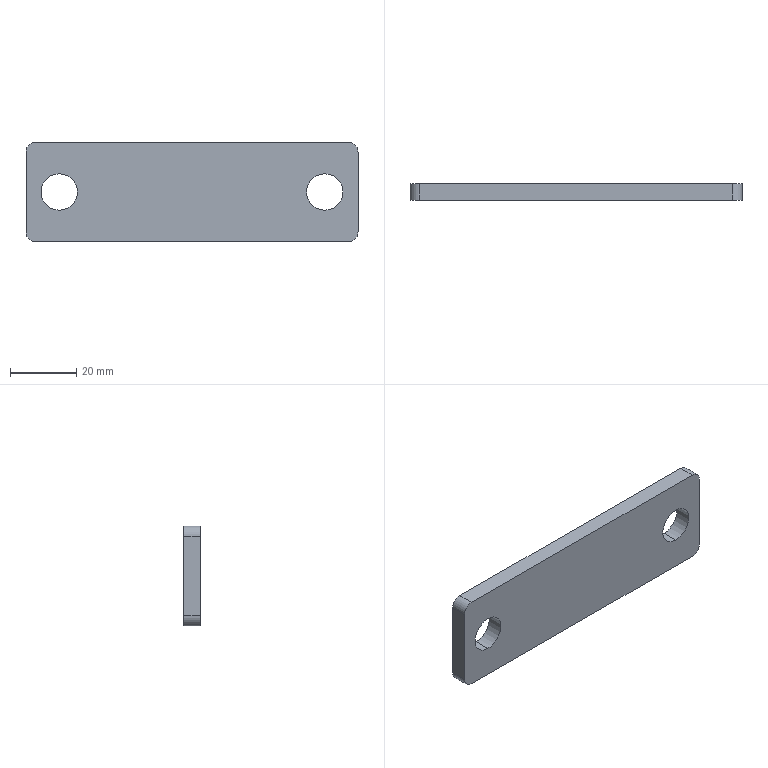Part | SolidWorks | features Extrusion 1, Fillet 1, ICE 1 | 1 solid | 14 faces | box 100 x 5 x 30 mm | volume 14011 mm3 | cylinder 8 | plane 6 | commonest cylinder face diameters 6 x4 11 x4
STEP:
#1=CARTESIAN_POINT('',(-40.,0.,5.5));
#2=VERTEX_POINT('',#1);
#3=CARTESIAN_POINT('',(-40.,0.,-5.5));
#4=VERTEX_POINT('',#3);
#5=CARTESIAN_POINT('',(-40.,0.,0.));
#6=DIRECTION('',(0.,-1.,0.));
#7=DIRECTION('',(0.,0.,-1.));
#8=AXIS2_PLACEMENT_3D('',#5,#6,#7);
#9=CIRCLE('',#8,5.5);
#10=EDGE_CURVE('',#2,#4,#9,.T.);
#11=ORIENTED_EDGE('',*,*,#10,.T.);
#12=CARTESIAN_POINT('',(-40.,5.,-5.5));
#13=VERTEX_POINT('',#12);
#14=CARTESIAN_POINT('',(-40.,-5.,-5.5));
#15=DIRECTION('',(0.,1.,0.));
#16=VECTOR('',#15,1000.);
#17=LINE('',#14,#16);
#18=EDGE_CURVE('',#4,#13,#17,.T.);
#19=ORIENTED_EDGE('',*,*,#18,.T.);
#20=CARTESIAN_POINT('',(-40.,5.,5.5));
#21=VERTEX_POINT('',#20);
#22=CARTESIAN_POINT('',(-40.,5.,0.));
#23=DIRECTION('',(0.,1.,0.));
#24=DIRECTION('',(0.,0.,1.));
#25=AXIS2_PLACEMENT_3D('',#22,#23,#24);
#26=CIRCLE('',#25,5.5);
#27=EDGE_CURVE('',#13,#21,#26,.T.);
#28=ORIENTED_EDGE('',*,*,#27,.T.);
#29=CARTESIAN_POINT('',(-40.,-5.,5.5));
#30=DIRECTION('',(0.,1.,0.));
#31=VECTOR('',#30,1000.);
#32=LINE('',#29,#31);
#33=EDGE_CURVE('',#2,#21,#32,.T.);
#34=ORIENTED_EDGE('',*,*,#33,.F.);
#35=EDGE_LOOP('',(#11,#19,#28,#34));
#36=FACE_OUTER_BOUND('',#35,.T.);
#37=CARTESIAN_POINT('',(-40.,-5.,0.));
#38=DIRECTION('',(0.,1.,0.));
#39=DIRECTION('',(0.,0.,1.));
#40=AXIS2_PLACEMENT_3D('',#37,#38,#39);
#41=CYLINDRICAL_SURFACE('',#40,5.5);
#42=ADVANCED_FACE('',(#36),#41,.F.);
#43=CARTESIAN_POINT('',(40.,0.,5.5));
#44=VERTEX_POINT('',#43);
#45=CARTESIAN_POINT('',(40.,0.,-5.5));
#46=VERTEX_POINT('',#45);
#47=CARTESIAN_POINT('',(40.,0.,0.));
#48=DIRECTION('',(0.,-1.,0.));
#49=DIRECTION('',(0.,0.,-1.));
#50=AXIS2_PLACEMENT_3D('',#47,#48,#49);
#51=CIRCLE('',#50,5.5);
#52=EDGE_CURVE('',#44,#46,#51,.T.);
#53=ORIENTED_EDGE('',*,*,#52,.T.);
#54=CARTESIAN_POINT('',(40.,5.,-5.5));
#55=VERTEX_POINT('',#54);
#56=CARTESIAN_POINT('',(40.,-5.,-5.5));
#57=DIRECTION('',(0.,1.,0.));
#58=VECTOR('',#57,1000.);
#59=LINE('',#56,#58);
#60=EDGE_CURVE('',#46,#55,#59,.T.);
#61=ORIENTED_EDGE('',*,*,#60,.T.);
#62=CARTESIAN_POINT('',(40.,5.,5.5));
#63=VERTEX_POINT('',#62);
#64=CARTESIAN_POINT('',(40.,5.,0.));
#65=DIRECTION('',(0.,1.,0.));
#66=DIRECTION('',(0.,0.,1.));
#67=AXIS2_PLACEMENT_3D('',#64,#65,#66);
#68=CIRCLE('',#67,5.5);
#69=EDGE_CURVE('',#55,#63,#68,.T.);
#70=ORIENTED_EDGE('',*,*,#69,.T.);
#71=CARTESIAN_POINT('',(40.,-5.,5.5));
#72=DIRECTION('',(0.,1.,0.));
#73=VECTOR('',#72,1000.);
#74=LINE('',#71,#73);
#75=EDGE_CURVE('',#44,#63,#74,.T.);
#76=ORIENTED_EDGE('',*,*,#75,.F.);
#77=EDGE_LOOP('',(#53,#61,#70,#76));
#78=FACE_OUTER_BOUND('',#77,.T.);
#79=CARTESIAN_POINT('',(40.,-5.,0.));
#80=DIRECTION('',(0.,1.,0.));
#81=DIRECTION('',(0.,0.,1.));
#82=AXIS2_PLACEMENT_3D('',#79,#80,#81);
#83=CYLINDRICAL_SURFACE('',#82,5.5);
#84=ADVANCED_FACE('',(#78),#83,.F.);
#85=CARTESIAN_POINT('',(50.,5.,12.));
#86=VERTEX_POINT('',#85);
#87=CARTESIAN_POINT('',(50.,5.,-12.));
#88=VERTEX_POINT('',#87);
#89=CARTESIAN_POINT('',(50.,5.,15.));
#90=DIRECTION('',(0.,0.,-1.));
#91=VECTOR('',#90,1000.);
#92=LINE('',#89,#91);
#93=EDGE_CURVE('',#86,#88,#92,.T.);
#94=ORIENTED_EDGE('',*,*,#93,.F.);
#95=CARTESIAN_POINT('',(50.,0.,12.));
#96=VERTEX_POINT('',#95);
#97=CARTESIAN_POINT('',(50.,5.,12.));
#98=DIRECTION('',(0.,-1.,0.));
#99=VECTOR('',#98,1000.);
#100=LINE('',#97,#99);
#101=EDGE_CURVE('',#86,#96,#100,.T.);
#102=ORIENTED_EDGE('',*,*,#101,.T.);
#103=CARTESIAN_POINT('',(50.,0.,-12.));
#104=VERTEX_POINT('',#103);
#105=CARTESIAN_POINT('',(50.,0.,15.));
#106=DIRECTION('',(0.,0.,-1.));
#107=VECTOR('',#106,1000.);
#108=LINE('',#105,#107);
#109=EDGE_CURVE('',#96,#104,#108,.T.);
#110=ORIENTED_EDGE('',*,*,#109,.T.);
#111=CARTESIAN_POINT('',(50.,5.,-12.));
#112=DIRECTION('',(0.,1.,0.));
#113=VECTOR('',#112,1000.);
#114=LINE('',#111,#113);
#115=EDGE_CURVE('',#104,#88,#114,.T.);
#116=ORIENTED_EDGE('',*,*,#115,.T.);
#117=EDGE_LOOP('',(#94,#102,#110,#116));
#118=FACE_OUTER_BOUND('',#117,.T.);
#119=CARTESIAN_POINT('',(50.,5.,15.));
#120=DIRECTION('',(-1.,0.,0.));
#121=DIRECTION('',(0.,0.,1.));
#122=AXIS2_PLACEMENT_3D('',#119,#120,#121);
#123=PLANE('',#122);
#124=ADVANCED_FACE('',(#118),#123,.F.);
#125=CARTESIAN_POINT('',(47.,5.,-15.));
#126=VERTEX_POINT('',#125);
#127=CARTESIAN_POINT('',(-47.,5.,-15.));
#128=VERTEX_POINT('',#127);
#129=CARTESIAN_POINT('',(-50.,5.,-15.));
#130=DIRECTION('',(-1.,0.,0.));
#131=VECTOR('',#130,1000.);
#132=LINE('',#129,#131);
#133=EDGE_CURVE('',#126,#128,#132,.T.);
#134=ORIENTED_EDGE('',*,*,#133,.F.);
#135=CARTESIAN_POINT('',(47.,0.,-15.));
#136=VERTEX_POINT('',#135);
#137=CARTESIAN_POINT('',(47.,5.,-15.));
#138=DIRECTION('',(0.,-1.,0.));
#139=VECTOR('',#138,1000.);
#140=LINE('',#137,#139);
#141=EDGE_CURVE('',#126,#136,#140,.T.);
#142=ORIENTED_EDGE('',*,*,#141,.T.);
#143=CARTESIAN_POINT('',(-47.,0.,-15.));
#144=VERTEX_POINT('',#143);
#145=CARTESIAN_POINT('',(-50.,0.,-15.));
#146=DIRECTION('',(-1.,0.,0.));
#147=VECTOR('',#146,1000.);
#148=LINE('',#145,#147);
#149=EDGE_CURVE('',#136,#144,#148,.T.);
#150=ORIENTED_EDGE('',*,*,#149,.T.);
#151=CARTESIAN_POINT('',(-47.,5.,-15.));
#152=DIRECTION('',(0.,1.,0.));
#153=VECTOR('',#152,1000.);
#154=LINE('',#151,#153);
#155=EDGE_CURVE('',#144,#128,#154,.T.);
#156=ORIENTED_EDGE('',*,*,#155,.T.);
#157=EDGE_LOOP('',(#134,#142,#150,#156));
#158=FACE_OUTER_BOUND('',#157,.T.);
#159=CARTESIAN_POINT('',(-50.,5.,-15.));
#160=DIRECTION('',(0.,0.,1.));
#161=DIRECTION('',(1.,0.,0.));
#162=AXIS2_PLACEMENT_3D('',#159,#160,#161);
#163=PLANE('',#162);
#164=ADVANCED_FACE('',(#158),#163,.F.);
#165=CARTESIAN_POINT('',(-50.,5.,-12.));
#166=VERTEX_POINT('',#165);
#167=CARTESIAN_POINT('',(-50.,5.,12.));
#168=VERTEX_POINT('',#167);
#169=CARTESIAN_POINT('',(-50.,5.,15.));
#170=DIRECTION('',(0.,0.,1.));
#171=VECTOR('',#170,1000.);
#172=LINE('',#169,#171);
#173=EDGE_CURVE('',#166,#168,#172,.T.);
#174=ORIENTED_EDGE('',*,*,#173,.F.);
#175=CARTESIAN_POINT('',(-50.,0.,-12.));
#176=VERTEX_POINT('',#175);
#177=CARTESIAN_POINT('',(-50.,5.,-12.));
#178=DIRECTION('',(0.,-1.,0.));
#179=VECTOR('',#178,1000.);
#180=LINE('',#177,#179);
#181=EDGE_CURVE('',#166,#176,#180,.T.);
#182=ORIENTED_EDGE('',*,*,#181,.T.);
#183=CARTESIAN_POINT('',(-50.,0.,12.));
#184=VERTEX_POINT('',#183);
#185=CARTESIAN_POINT('',(-50.,0.,15.));
#186=DIRECTION('',(0.,0.,1.));
#187=VECTOR('',#186,1000.);
#188=LINE('',#185,#187);
#189=EDGE_CURVE('',#176,#184,#188,.T.);
#190=ORIENTED_EDGE('',*,*,#189,.T.);
#191=CARTESIAN_POINT('',(-50.,5.,12.));
#192=DIRECTION('',(0.,1.,0.));
#193=VECTOR('',#192,1000.);
#194=LINE('',#191,#193);
#195=EDGE_CURVE('',#184,#168,#194,.T.);
#196=ORIENTED_EDGE('',*,*,#195,.T.);
#197=EDGE_LOOP('',(#174,#182,#190,#196));
#198=FACE_OUTER_BOUND('',#197,.T.);
#199=CARTESIAN_POINT('',(-50.,5.,15.));
#200=DIRECTION('',(1.,0.,0.));
#201=DIRECTION('',(0.,0.,-1.));
#202=AXIS2_PLACEMENT_3D('',#199,#200,#201);
#203=PLANE('',#202);
#204=ADVANCED_FACE('',(#198),#203,.F.);
#205=CARTESIAN_POINT('',(-47.,0.,15.));
#206=VERTEX_POINT('',#205);
#207=CARTESIAN_POINT('',(47.,0.,15.));
#208=VERTEX_POINT('',#207);
#209=CARTESIAN_POINT('',(-50.,0.,15.));
#210=DIRECTION('',(1.,0.,0.));
#211=VECTOR('',#210,1000.);
#212=LINE('',#209,#211);
#213=EDGE_CURVE('',#206,#208,#212,.T.);
#214=ORIENTED_EDGE('',*,*,#213,.T.);
#215=CARTESIAN_POINT('',(47.,5.,15.));
#216=VERTEX_POINT('',#215);
#217=CARTESIAN_POINT('',(47.,5.,15.));
#218=DIRECTION('',(0.,1.,0.));
#219=VECTOR('',#218,1000.);
#220=LINE('',#217,#219);
#221=EDGE_CURVE('',#208,#216,#220,.T.);
#222=ORIENTED_EDGE('',*,*,#221,.T.);
#223=CARTESIAN_POINT('',(-47.,5.,15.));
#224=VERTEX_POINT('',#223);
#225=CARTESIAN_POINT('',(-50.,5.,15.));
#226=DIRECTION('',(1.,0.,0.));
#227=VECTOR('',#226,1000.);
#228=LINE('',#225,#227);
#229=EDGE_CURVE('',#224,#216,#228,.T.);
#230=ORIENTED_EDGE('',*,*,#229,.F.);
#231=CARTESIAN_POINT('',(-47.,5.,15.));
#232=DIRECTION('',(0.,-1.,0.));
#233=VECTOR('',#232,1000.);
#234=LINE('',#231,#233);
#235=EDGE_CURVE('',#224,#206,#234,.T.);
#236=ORIENTED_EDGE('',*,*,#235,.T.);
#237=EDGE_LOOP('',(#214,#222,#230,#236));
#238=FACE_OUTER_BOUND('',#237,.T.);
#239=CARTESIAN_POINT('',(-50.,5.,15.));
#240=DIRECTION('',(0.,0.,-1.));
#241=DIRECTION('',(-1.,0.,0.));
#242=AXIS2_PLACEMENT_3D('',#239,#240,#241);
#243=PLANE('',#242);
#244=ADVANCED_FACE('',(#238),#243,.F.);
#245=CARTESIAN_POINT('',(-40.,5.,0.));
#246=DIRECTION('',(0.,1.,0.));
#247=DIRECTION('',(0.,0.,1.));
#248=AXIS2_PLACEMENT_3D('',#245,#246,#247);
#249=CIRCLE('',#248,5.5);
#250=EDGE_CURVE('',#21,#13,#249,.T.);
#251=ORIENTED_EDGE('',*,*,#250,.F.);
#252=ORIENTED_EDGE('',*,*,#27,.F.);
#253=EDGE_LOOP('',(#251,#252));
#254=FACE_BOUND('',#253,.T.);
#255=CARTESIAN_POINT('',(40.,5.,0.));
#256=DIRECTION('',(0.,1.,0.));
#257=DIRECTION('',(0.,0.,1.));
#258=AXIS2_PLACEMENT_3D('',#255,#256,#257);
#259=CIRCLE('',#258,5.5);
#260=EDGE_CURVE('',#63,#55,#259,.T.);
#261=ORIENTED_EDGE('',*,*,#260,.F.);
#262=ORIENTED_EDGE('',*,*,#69,.F.);
#263=EDGE_LOOP('',(#261,#262));
#264=FACE_BOUND('',#263,.T.);
#265=ORIENTED_EDGE('',*,*,#229,.T.);
#266=CARTESIAN_POINT('',(47.,5.,12.));
#267=DIRECTION('',(0.,1.,0.));
#268=DIRECTION('',(0.,0.,-1.));
#269=AXIS2_PLACEMENT_3D('',#266,#267,#268);
#270=CIRCLE('',#269,3.);
#271=EDGE_CURVE('',#216,#86,#270,.T.);
#272=ORIENTED_EDGE('',*,*,#271,.T.);
#273=ORIENTED_EDGE('',*,*,#93,.T.);
#274=CARTESIAN_POINT('',(47.,5.,-12.));
#275=DIRECTION('',(0.,1.,0.));
#276=DIRECTION('',(0.,0.,-1.));
#277=AXIS2_PLACEMENT_3D('',#274,#275,#276);
#278=CIRCLE('',#277,3.);
#279=EDGE_CURVE('',#88,#126,#278,.T.);
#280=ORIENTED_EDGE('',*,*,#279,.T.);
#281=ORIENTED_EDGE('',*,*,#133,.T.);
#282=CARTESIAN_POINT('',(-47.,5.,-12.));
#283=DIRECTION('',(0.,1.,0.));
#284=DIRECTION('',(0.,0.,-1.));
#285=AXIS2_PLACEMENT_3D('',#282,#283,#284);
#286=CIRCLE('',#285,3.);
#287=EDGE_CURVE('',#128,#166,#286,.T.);
#288=ORIENTED_EDGE('',*,*,#287,.T.);
#289=ORIENTED_EDGE('',*,*,#173,.T.);
#290=CARTESIAN_POINT('',(-47.,5.,12.));
#291=DIRECTION('',(0.,1.,0.));
#292=DIRECTION('',(0.,0.,-1.));
#293=AXIS2_PLACEMENT_3D('',#290,#291,#292);
#294=CIRCLE('',#293,3.);
#295=EDGE_CURVE('',#168,#224,#294,.T.);
#296=ORIENTED_EDGE('',*,*,#295,.T.);
#297=EDGE_LOOP('',(#265,#272,#273,#280,#281,#288,#289,#296));
#298=FACE_OUTER_BOUND('',#297,.T.);
#299=CARTESIAN_POINT('',(0.,5.,0.));
#300=DIRECTION('',(0.,-1.,0.));
#301=DIRECTION('',(0.,0.,-1.));
#302=AXIS2_PLACEMENT_3D('',#299,#300,#301);
#303=PLANE('',#302);
#304=ADVANCED_FACE('',(#254,#264,#298),#303,.F.);
#305=ORIENTED_EDGE('',*,*,#10,.F.);
#306=CARTESIAN_POINT('',(-40.,0.,0.));
#307=DIRECTION('',(0.,-1.,0.));
#308=DIRECTION('',(0.,0.,-1.));
#309=AXIS2_PLACEMENT_3D('',#306,#307,#308);
#310=CIRCLE('',#309,5.5);
#311=EDGE_CURVE('',#4,#2,#310,.T.);
#312=ORIENTED_EDGE('',*,*,#311,.F.);
#313=EDGE_LOOP('',(#305,#312));
#314=FACE_BOUND('',#313,.T.);
#315=ORIENTED_EDGE('',*,*,#52,.F.);
#316=CARTESIAN_POINT('',(40.,0.,0.));
#317=DIRECTION('',(0.,-1.,0.));
#318=DIRECTION('',(0.,0.,-1.));
#319=AXIS2_PLACEMENT_3D('',#316,#317,#318);
#320=CIRCLE('',#319,5.5);
#321=EDGE_CURVE('',#46,#44,#320,.T.);
#322=ORIENTED_EDGE('',*,*,#321,.F.);
#323=EDGE_LOOP('',(#315,#322));
#324=FACE_BOUND('',#323,.T.);
#325=ORIENTED_EDGE('',*,*,#109,.F.);
#326=CARTESIAN_POINT('',(47.,0.,12.));
#327=DIRECTION('',(0.,-1.,0.));
#328=DIRECTION('',(0.,0.,-1.));
#329=AXIS2_PLACEMENT_3D('',#326,#327,#328);
#330=CIRCLE('',#329,3.);
#331=EDGE_CURVE('',#96,#208,#330,.T.);
#332=ORIENTED_EDGE('',*,*,#331,.T.);
#333=ORIENTED_EDGE('',*,*,#213,.F.);
#334=CARTESIAN_POINT('',(-47.,0.,12.));
#335=DIRECTION('',(0.,-1.,0.));
#336=DIRECTION('',(0.,0.,-1.));
#337=AXIS2_PLACEMENT_3D('',#334,#335,#336);
#338=CIRCLE('',#337,3.);
#339=EDGE_CURVE('',#206,#184,#338,.T.);
#340=ORIENTED_EDGE('',*,*,#339,.T.);
#341=ORIENTED_EDGE('',*,*,#189,.F.);
#342=CARTESIAN_POINT('',(-47.,0.,-12.));
#343=DIRECTION('',(0.,-1.,0.));
#344=DIRECTION('',(0.,0.,-1.));
#345=AXIS2_PLACEMENT_3D('',#342,#343,#344);
#346=CIRCLE('',#345,3.);
#347=EDGE_CURVE('',#176,#144,#346,.T.);
#348=ORIENTED_EDGE('',*,*,#347,.T.);
#349=ORIENTED_EDGE('',*,*,#149,.F.);
#350=CARTESIAN_POINT('',(47.,0.,-12.));
#351=DIRECTION('',(0.,-1.,0.));
#352=DIRECTION('',(0.,0.,-1.));
#353=AXIS2_PLACEMENT_3D('',#350,#351,#352);
#354=CIRCLE('',#353,3.);
#355=EDGE_CURVE('',#136,#104,#354,.T.);
#356=ORIENTED_EDGE('',*,*,#355,.T.);
#357=EDGE_LOOP('',(#325,#332,#333,#340,#341,#348,#349,#356));
#358=FACE_OUTER_BOUND('',#357,.T.);
#359=CARTESIAN_POINT('',(0.,0.,0.));
#360=DIRECTION('',(0.,-1.,0.));
#361=DIRECTION('',(0.,0.,-1.));
#362=AXIS2_PLACEMENT_3D('',#359,#360,#361);
#363=PLANE('',#362);
#364=ADVANCED_FACE('',(#314,#324,#358),#363,.T.);
#365=ORIENTED_EDGE('',*,*,#271,.F.);
#366=ORIENTED_EDGE('',*,*,#221,.F.);
#367=ORIENTED_EDGE('',*,*,#331,.F.);
#368=ORIENTED_EDGE('',*,*,#101,.F.);
#369=EDGE_LOOP('',(#365,#366,#367,#368));
#370=FACE_OUTER_BOUND('',#369,.T.);
#371=CARTESIAN_POINT('',(47.,5.,12.));
#372=DIRECTION('',(0.,-1.,0.));
#373=DIRECTION('',(0.,0.,-1.));
#374=AXIS2_PLACEMENT_3D('',#371,#372,#373);
#375=CYLINDRICAL_SURFACE('',#374,3.);
#376=ADVANCED_FACE('',(#370),#375,.T.);
#377=ORIENTED_EDGE('',*,*,#279,.F.);
#378=ORIENTED_EDGE('',*,*,#115,.F.);
#379=ORIENTED_EDGE('',*,*,#355,.F.);
#380=ORIENTED_EDGE('',*,*,#141,.F.);
#381=EDGE_LOOP('',(#377,#378,#379,#380));
#382=FACE_OUTER_BOUND('',#381,.T.);
#383=CARTESIAN_POINT('',(47.,5.,-12.));
#384=DIRECTION('',(0.,-1.,0.));
#385=DIRECTION('',(0.,0.,-1.));
#386=AXIS2_PLACEMENT_3D('',#383,#384,#385);
#387=CYLINDRICAL_SURFACE('',#386,3.);
#388=ADVANCED_FACE('',(#382),#387,.T.);
#389=ORIENTED_EDGE('',*,*,#287,.F.);
#390=ORIENTED_EDGE('',*,*,#155,.F.);
#391=ORIENTED_EDGE('',*,*,#347,.F.);
#392=ORIENTED_EDGE('',*,*,#181,.F.);
#393=EDGE_LOOP('',(#389,#390,#391,#392));
#394=FACE_OUTER_BOUND('',#393,.T.);
#395=CARTESIAN_POINT('',(-47.,5.,-12.));
#396=DIRECTION('',(0.,-1.,0.));
#397=DIRECTION('',(0.,0.,-1.));
#398=AXIS2_PLACEMENT_3D('',#395,#396,#397);
#399=CYLINDRICAL_SURFACE('',#398,3.);
#400=ADVANCED_FACE('',(#394),#399,.T.);
#401=ORIENTED_EDGE('',*,*,#295,.F.);
#402=ORIENTED_EDGE('',*,*,#195,.F.);
#403=ORIENTED_EDGE('',*,*,#339,.F.);
#404=ORIENTED_EDGE('',*,*,#235,.F.);
#405=EDGE_LOOP('',(#401,#402,#403,#404));
#406=FACE_OUTER_BOUND('',#405,.T.);
#407=CARTESIAN_POINT('',(-47.,5.,12.));
#408=DIRECTION('',(0.,-1.,0.));
#409=DIRECTION('',(0.,0.,-1.));
#410=AXIS2_PLACEMENT_3D('',#407,#408,#409);
#411=CYLINDRICAL_SURFACE('',#410,3.);
#412=ADVANCED_FACE('',(#406),#411,.T.);
#413=ORIENTED_EDGE('',*,*,#60,.F.);
#414=ORIENTED_EDGE('',*,*,#321,.T.);
#415=ORIENTED_EDGE('',*,*,#75,.T.);
#416=ORIENTED_EDGE('',*,*,#260,.T.);
#417=EDGE_LOOP('',(#413,#414,#415,#416));
#418=FACE_OUTER_BOUND('',#417,.T.);
#419=CARTESIAN_POINT('',(40.,-5.,0.));
#420=DIRECTION('',(0.,1.,0.));
#421=DIRECTION('',(0.,0.,1.));
#422=AXIS2_PLACEMENT_3D('',#419,#420,#421);
#423=CYLINDRICAL_SURFACE('',#422,5.5);
#424=ADVANCED_FACE('',(#418),#423,.F.);
#425=ORIENTED_EDGE('',*,*,#18,.F.);
#426=ORIENTED_EDGE('',*,*,#311,.T.);
#427=ORIENTED_EDGE('',*,*,#33,.T.);
#428=ORIENTED_EDGE('',*,*,#250,.T.);
#429=EDGE_LOOP('',(#425,#426,#427,#428));
#430=FACE_OUTER_BOUND('',#429,.T.);
#431=CARTESIAN_POINT('',(-40.,-5.,0.));
#432=DIRECTION('',(0.,1.,0.));
#433=DIRECTION('',(0.,0.,1.));
#434=AXIS2_PLACEMENT_3D('',#431,#432,#433);
#435=CYLINDRICAL_SURFACE('',#434,5.5);
#436=ADVANCED_FACE('',(#430),#435,.F.);
#437=CLOSED_SHELL('',(#42,#84,#124,#164,#204,#244,#304,#364,#376,#388,#400,#412,#424,#436));
#438=MANIFOLD_SOLID_BREP('',#437);
#439=CARTESIAN_POINT('',(0.,0.,0.));
#440=DIRECTION('',(0.,0.,1.));
#441=DIRECTION('',(1.,0.,0.));
#442=AXIS2_PLACEMENT_3D('',#439,#440,#441);
#443=(LENGTH_UNIT()NAMED_UNIT(*)SI_UNIT(.MILLI.,.METRE.));
#444=UNCERTAINTY_MEASURE_WITH_UNIT(LENGTH_MEASURE(0.00001),#443,'','');
#445=(NAMED_UNIT(*)PLANE_ANGLE_UNIT()SI_UNIT($,.RADIAN.));
#446=(NAMED_UNIT(*)SI_UNIT($,.STERADIAN.)SOLID_ANGLE_UNIT());
#447=(GEOMETRIC_REPRESENTATION_CONTEXT(3)GLOBAL_UNCERTAINTY_ASSIGNED_CONTEXT((#444))GLOBAL_UNIT_ASSIGNED_CONTEXT((#443,#445,#446))REPRESENTATION_CONTEXT('',''));
#448=ADVANCED_BREP_SHAPE_REPRESENTATION('',(#438,#442),#447);